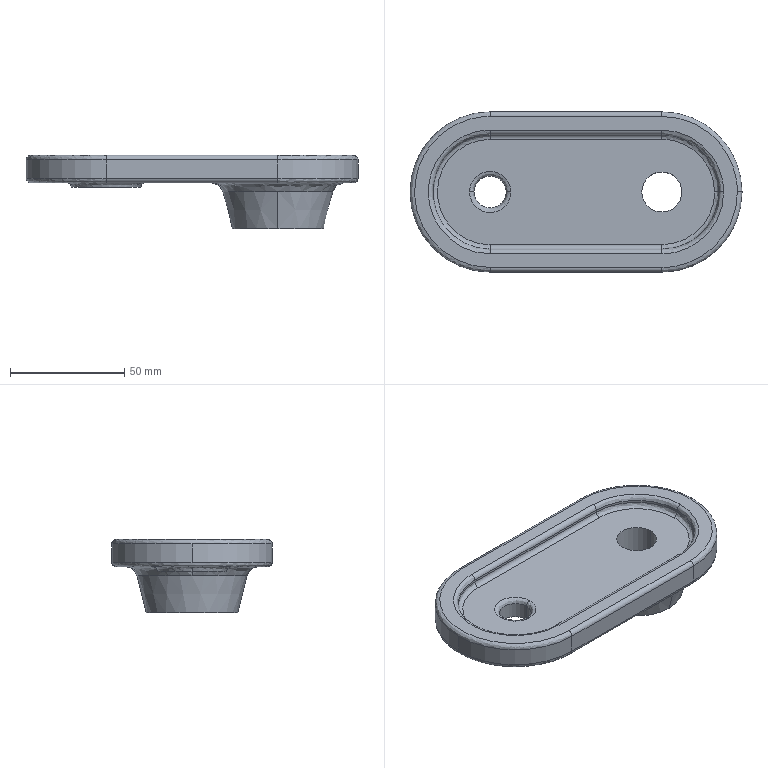Part | STEP file | 1 solid | 47 faces | box 145 x 70 x 32 mm | volume 105996 mm3 | cylinder 18 | spline 18 | plane 9 | cone 2 | commonest cylinder face diameters 4 x8 50 x3 70 x3 14 x2 17.5 x2